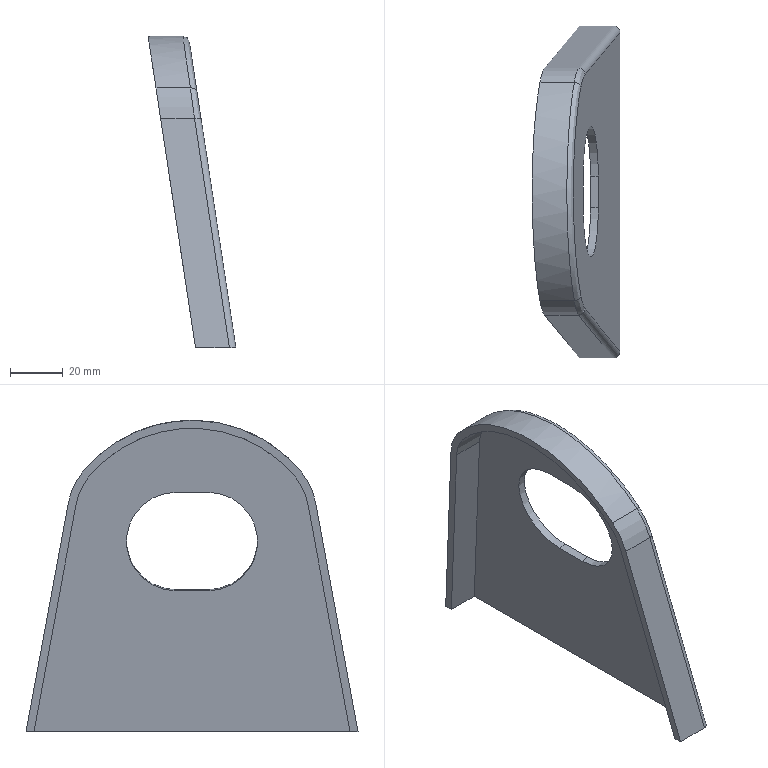Part | STEP file | 1-57.5 | 1 solid | 23 faces | box 33.418 x 126.49 x 118.588 mm | volume 41627 mm3 | plane 10 | cylinder 10 | spline 3 | commonest cylinder face diameters 5 x2 38 x2 45 x2 51 x2 102 x1 108 x1